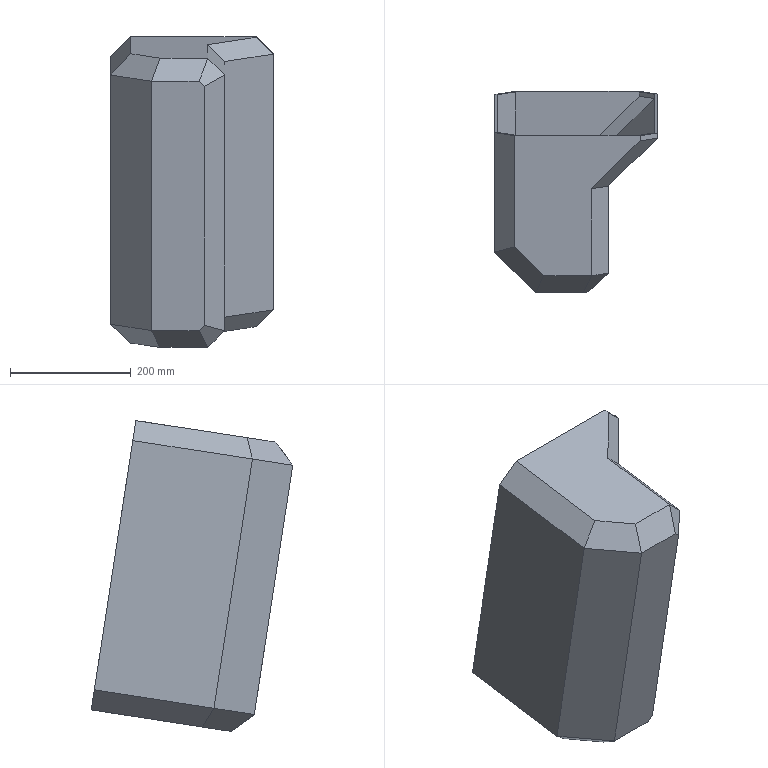Part | SolidWorks | features BaseBody 1 | 1 solid | 47 faces | box 269.204 x 333.071 x 514.026 mm | volume 1628567 mm3 | plane 47
STEP:
#1=CARTESIAN_POINT('',(-323.449,318.377,-419.092));
#2=VERTEX_POINT('',#1);
#3=CARTESIAN_POINT('',(-323.449,175.26,-441.176));
#4=VERTEX_POINT('',#3);
#5=CARTESIAN_POINT('',(-323.449,318.377,-419.092));
#6=DIRECTION('',(0.,-0.9883,-0.1525));
#7=VECTOR('',#6,1000.);
#8=LINE('',#5,#7);
#9=EDGE_CURVE('',#2,#4,#8,.T.);
#10=ORIENTED_EDGE('',*,*,#9,.F.);
#11=CARTESIAN_POINT('',(-352.149,314.001,-390.728));
#12=VERTEX_POINT('',#11);
#13=CARTESIAN_POINT('',(-323.449,318.377,-419.092));
#14=DIRECTION('',(-0.7071,-0.1078,0.6988));
#15=VECTOR('',#14,1000.);
#16=LINE('',#13,#15);
#17=EDGE_CURVE('',#2,#12,#16,.T.);
#18=ORIENTED_EDGE('',*,*,#17,.T.);
#19=CARTESIAN_POINT('',(-352.149,170.489,-412.872));
#20=VERTEX_POINT('',#19);
#21=CARTESIAN_POINT('',(-352.149,314.001,-390.728));
#22=DIRECTION('',(0.,-0.9883,-0.1525));
#23=VECTOR('',#22,1000.);
#24=LINE('',#21,#23);
#25=EDGE_CURVE('',#12,#20,#24,.T.);
#26=ORIENTED_EDGE('',*,*,#25,.T.);
#27=CARTESIAN_POINT('',(-351.829,170.222,-413.237));
#28=VERTEX_POINT('',#27);
#29=CARTESIAN_POINT('',(-352.149,170.489,-412.872));
#30=DIRECTION('',(0.5774,-0.4826,-0.6586));
#31=VECTOR('',#30,1000.);
#32=LINE('',#29,#31);
#33=EDGE_CURVE('',#20,#28,#32,.T.);
#34=ORIENTED_EDGE('',*,*,#33,.T.);
#35=CARTESIAN_POINT('',(-324.165,174.442,-440.577));
#36=VERTEX_POINT('',#35);
#37=CARTESIAN_POINT('',(-351.829,170.222,-413.237));
#38=DIRECTION('',(0.7071,0.1079,-0.6988));
#39=VECTOR('',#38,1000.);
#40=LINE('',#37,#39);
#41=EDGE_CURVE('',#28,#36,#40,.T.);
#42=ORIENTED_EDGE('',*,*,#41,.T.);
#43=CARTESIAN_POINT('',(-323.449,175.26,-441.176));
#44=DIRECTION('',(-0.5774,-0.6586,0.4826));
#45=VECTOR('',#44,1000.);
#46=LINE('',#43,#45);
#47=EDGE_CURVE('',#4,#36,#46,.T.);
#48=ORIENTED_EDGE('',*,*,#47,.F.);
#49=EDGE_LOOP('',(#10,#18,#26,#34,#42,#48));
#50=FACE_OUTER_BOUND('',#49,.T.);
#51=CARTESIAN_POINT('',(-363.649,121.114,-408.855));
#52=DIRECTION('',(-0.7071,0.1078,-0.6988));
#53=DIRECTION('',(-0.7029,0.,0.7113));
#54=AXIS2_PLACEMENT_3D('',#51,#52,#53);
#55=PLANE('',#54);
#56=ADVANCED_FACE('',(#50),#55,.F.);
#57=CARTESIAN_POINT('',(-324.165,239.716,-863.606));
#58=VERTEX_POINT('',#57);
#59=CARTESIAN_POINT('',(-323.449,240.315,-862.788));
#60=VERTEX_POINT('',#59);
#61=CARTESIAN_POINT('',(-324.165,239.716,-863.606));
#62=DIRECTION('',(0.5774,0.4826,0.6586));
#63=VECTOR('',#62,1000.);
#64=LINE('',#61,#63);
#65=EDGE_CURVE('',#58,#60,#64,.T.);
#66=ORIENTED_EDGE('',*,*,#65,.T.);
#67=CARTESIAN_POINT('',(-323.449,175.26,-441.176));
#68=DIRECTION('',(0.,0.1525,-0.9883));
#69=VECTOR('',#68,1000.);
#70=LINE('',#67,#69);
#71=EDGE_CURVE('',#4,#60,#70,.T.);
#72=ORIENTED_EDGE('',*,*,#71,.F.);
#73=ORIENTED_EDGE('',*,*,#47,.T.);
#74=CARTESIAN_POINT('',(-357.348,143.81,-459.65));
#75=VERTEX_POINT('',#74);
#76=CARTESIAN_POINT('',(-357.348,143.81,-459.65));
#77=DIRECTION('',(0.6769,0.6249,0.3891));
#78=VECTOR('',#77,1000.);
#79=LINE('',#76,#78);
#80=EDGE_CURVE('',#75,#36,#79,.T.);
#81=ORIENTED_EDGE('',*,*,#80,.F.);
#82=CARTESIAN_POINT('',(-357.348,204.76,-854.653));
#83=VERTEX_POINT('',#82);
#84=CARTESIAN_POINT('',(-357.348,204.76,-854.653));
#85=DIRECTION('',(0.,-0.1525,0.9883));
#86=VECTOR('',#85,1000.);
#87=LINE('',#84,#86);
#88=EDGE_CURVE('',#83,#75,#87,.T.);
#89=ORIENTED_EDGE('',*,*,#88,.F.);
#90=CARTESIAN_POINT('',(-357.348,204.76,-854.653));
#91=DIRECTION('',(0.6769,0.7131,-0.1826));
#92=VECTOR('',#91,1000.);
#93=LINE('',#90,#92);
#94=EDGE_CURVE('',#83,#58,#93,.T.);
#95=ORIENTED_EDGE('',*,*,#94,.T.);
#96=EDGE_LOOP('',(#66,#72,#73,#81,#89,#95));
#97=FACE_OUTER_BOUND('',#96,.T.);
#98=CARTESIAN_POINT('',(-321.336,164.858,-359.909));
#99=DIRECTION('',(-0.7071,0.6988,0.1078));
#100=DIRECTION('',(0.1508,0.,0.9886));
#101=AXIS2_PLACEMENT_3D('',#98,#99,#100);
#102=PLANE('',#101);
#103=ADVANCED_FACE('',(#97),#102,.F.);
#104=CARTESIAN_POINT('',(-366.009,206.081,-863.214));
#105=VERTEX_POINT('',#104);
#106=CARTESIAN_POINT('',(-351.829,243.933,-890.946));
#107=VERTEX_POINT('',#106);
#108=CARTESIAN_POINT('',(-366.009,206.081,-863.214));
#109=DIRECTION('',(0.2893,0.7722,-0.5657));
#110=VECTOR('',#109,1000.);
#111=LINE('',#108,#110);
#112=EDGE_CURVE('',#105,#107,#111,.T.);
#113=ORIENTED_EDGE('',*,*,#112,.T.);
#114=CARTESIAN_POINT('',(-324.165,239.716,-863.606));
#115=DIRECTION('',(-0.7071,0.1078,-0.6988));
#116=VECTOR('',#115,1000.);
#117=LINE('',#114,#116);
#118=EDGE_CURVE('',#58,#107,#117,.T.);
#119=ORIENTED_EDGE('',*,*,#118,.F.);
#120=ORIENTED_EDGE('',*,*,#94,.F.);
#121=CARTESIAN_POINT('',(-366.009,206.081,-863.214));
#122=DIRECTION('',(0.7071,-0.1078,0.6989));
#123=VECTOR('',#122,1000.);
#124=LINE('',#121,#123);
#125=EDGE_CURVE('',#105,#83,#124,.T.);
#126=ORIENTED_EDGE('',*,*,#125,.F.);
#127=EDGE_LOOP('',(#113,#119,#120,#126));
#128=FACE_OUTER_BOUND('',#127,.T.);
#129=CARTESIAN_POINT('',(-238.738,183.663,-734.28));
#130=DIRECTION('',(0.4977,-0.6262,-0.6002));
#131=DIRECTION('',(0.,0.692,-0.7219));
#132=AXIS2_PLACEMENT_3D('',#129,#130,#131);
#133=PLANE('',#132);
#134=ADVANCED_FACE('',(#128),#133,.T.);
#135=ORIENTED_EDGE('',*,*,#88,.T.);
#136=CARTESIAN_POINT('',(-366.009,142.489,-451.089));
#137=VERTEX_POINT('',#136);
#138=CARTESIAN_POINT('',(-357.348,143.81,-459.65));
#139=DIRECTION('',(-0.7071,-0.1078,0.6989));
#140=VECTOR('',#139,1000.);
#141=LINE('',#138,#140);
#142=EDGE_CURVE('',#75,#137,#141,.T.);
#143=ORIENTED_EDGE('',*,*,#142,.T.);
#144=CARTESIAN_POINT('',(-444.924,142.489,-451.089));
#145=VERTEX_POINT('',#144);
#146=CARTESIAN_POINT('',(-444.924,142.489,-451.089));
#147=DIRECTION('',(1.,0.,0.));
#148=VECTOR('',#147,1000.);
#149=LINE('',#146,#148);
#150=EDGE_CURVE('',#145,#137,#149,.T.);
#151=ORIENTED_EDGE('',*,*,#150,.F.);
#152=CARTESIAN_POINT('',(-444.924,206.081,-863.214));
#153=VERTEX_POINT('',#152);
#154=CARTESIAN_POINT('',(-444.924,142.489,-451.089));
#155=DIRECTION('',(0.,0.1525,-0.9883));
#156=VECTOR('',#155,1000.);
#157=LINE('',#154,#156);
#158=EDGE_CURVE('',#145,#153,#157,.T.);
#159=ORIENTED_EDGE('',*,*,#158,.T.);
#160=CARTESIAN_POINT('',(-366.009,206.081,-863.214));
#161=DIRECTION('',(-1.,0.,0.));
#162=VECTOR('',#161,1000.);
#163=LINE('',#160,#162);
#164=EDGE_CURVE('',#105,#153,#163,.T.);
#165=ORIENTED_EDGE('',*,*,#164,.F.);
#166=ORIENTED_EDGE('',*,*,#125,.T.);
#167=EDGE_LOOP('',(#135,#143,#151,#159,#165,#166));
#168=FACE_OUTER_BOUND('',#167,.T.);
#169=CARTESIAN_POINT('',(-335.294,177.166,-675.82));
#170=DIRECTION('',(0.,0.9883,0.1525));
#171=DIRECTION('',(1.,0.,0.));
#172=AXIS2_PLACEMENT_3D('',#169,#170,#171);
#173=PLANE('',#172);
#174=ADVANCED_FACE('',(#168),#173,.F.);
#175=ORIENTED_EDGE('',*,*,#164,.T.);
#176=CARTESIAN_POINT('',(-431.048,244.298,-891.213));
#177=VERTEX_POINT('',#176);
#178=CARTESIAN_POINT('',(-431.048,244.298,-891.213));
#179=DIRECTION('',(-0.2811,-0.7741,0.5672));
#180=VECTOR('',#179,1000.);
#181=LINE('',#178,#180);
#182=EDGE_CURVE('',#177,#153,#181,.T.);
#183=ORIENTED_EDGE('',*,*,#182,.F.);
#184=CARTESIAN_POINT('',(-352.149,244.298,-891.213));
#185=VERTEX_POINT('',#184);
#186=CARTESIAN_POINT('',(-431.048,244.298,-891.213));
#187=DIRECTION('',(1.,0.,0.));
#188=VECTOR('',#187,1000.);
#189=LINE('',#186,#188);
#190=EDGE_CURVE('',#177,#185,#189,.T.);
#191=ORIENTED_EDGE('',*,*,#190,.T.);
#192=CARTESIAN_POINT('',(-352.149,244.298,-891.213));
#193=DIRECTION('',(0.5774,-0.6586,0.4826));
#194=VECTOR('',#193,1000.);
#195=LINE('',#192,#194);
#196=EDGE_CURVE('',#185,#107,#195,.T.);
#197=ORIENTED_EDGE('',*,*,#196,.T.);
#198=ORIENTED_EDGE('',*,*,#112,.F.);
#199=EDGE_LOOP('',(#175,#183,#191,#197,#198));
#200=FACE_OUTER_BOUND('',#199,.T.);
#201=CARTESIAN_POINT('',(-444.924,206.081,-863.214));
#202=DIRECTION('',(0.,-0.591,-0.8067));
#203=DIRECTION('',(0.,-0.8067,0.591));
#204=AXIS2_PLACEMENT_3D('',#201,#202,#203);
#205=PLANE('',#204);
#206=ADVANCED_FACE('',(#200),#205,.T.);
#207=CARTESIAN_POINT('',(-352.149,387.809,-869.069));
#208=VERTEX_POINT('',#207);
#209=CARTESIAN_POINT('',(-352.149,244.298,-891.213));
#210=DIRECTION('',(0.,0.9883,0.1525));
#211=VECTOR('',#210,1000.);
#212=LINE('',#209,#211);
#213=EDGE_CURVE('',#185,#208,#212,.T.);
#214=ORIENTED_EDGE('',*,*,#213,.T.);
#215=CARTESIAN_POINT('',(-323.449,383.433,-840.705));
#216=VERTEX_POINT('',#215);
#217=CARTESIAN_POINT('',(-323.449,383.433,-840.705));
#218=DIRECTION('',(-0.7071,0.1078,-0.6988));
#219=VECTOR('',#218,1000.);
#220=LINE('',#217,#219);
#221=EDGE_CURVE('',#216,#208,#220,.T.);
#222=ORIENTED_EDGE('',*,*,#221,.F.);
#223=CARTESIAN_POINT('',(-323.449,383.433,-840.705));
#224=DIRECTION('',(0.,-0.9883,-0.1525));
#225=VECTOR('',#224,1000.);
#226=LINE('',#223,#225);
#227=EDGE_CURVE('',#216,#60,#226,.T.);
#228=ORIENTED_EDGE('',*,*,#227,.T.);
#229=ORIENTED_EDGE('',*,*,#65,.F.);
#230=ORIENTED_EDGE('',*,*,#118,.T.);
#231=ORIENTED_EDGE('',*,*,#196,.F.);
#232=EDGE_LOOP('',(#214,#222,#228,#229,#230,#231));
#233=FACE_OUTER_BOUND('',#232,.T.);
#234=CARTESIAN_POINT('',(-363.649,198.431,-909.927));
#235=DIRECTION('',(0.7071,0.1078,-0.6988));
#236=DIRECTION('',(0.,-0.9883,-0.1525));
#237=AXIS2_PLACEMENT_3D('',#234,#235,#236);
#238=PLANE('',#237);
#239=ADVANCED_FACE('',(#233),#238,.T.);
#240=ORIENTED_EDGE('',*,*,#227,.F.);
#241=CARTESIAN_POINT('',(-323.449,384.088,-841.185));
#242=VERTEX_POINT('',#241);
#243=CARTESIAN_POINT('',(-323.449,383.433,-840.705));
#244=DIRECTION('',(0.,0.8067,-0.591));
#245=VECTOR('',#244,1000.);
#246=LINE('',#243,#245);
#247=EDGE_CURVE('',#216,#242,#246,.T.);
#248=ORIENTED_EDGE('',*,*,#247,.T.);
#249=CARTESIAN_POINT('',(-323.449,318.857,-418.438));
#250=VERTEX_POINT('',#249);
#251=CARTESIAN_POINT('',(-323.449,384.088,-841.185));
#252=DIRECTION('',(0.,-0.1525,0.9883));
#253=VECTOR('',#252,1000.);
#254=LINE('',#251,#253);
#255=EDGE_CURVE('',#242,#250,#254,.T.);
#256=ORIENTED_EDGE('',*,*,#255,.T.);
#257=CARTESIAN_POINT('',(-323.449,318.377,-419.092));
#258=DIRECTION('',(0.,0.591,0.8067));
#259=VECTOR('',#258,1000.);
#260=LINE('',#257,#259);
#261=EDGE_CURVE('',#2,#250,#260,.T.);
#262=ORIENTED_EDGE('',*,*,#261,.F.);
#263=ORIENTED_EDGE('',*,*,#9,.T.);
#264=ORIENTED_EDGE('',*,*,#71,.T.);
#265=EDGE_LOOP('',(#240,#248,#256,#262,#263,#264));
#266=FACE_OUTER_BOUND('',#265,.T.);
#267=CARTESIAN_POINT('',(-323.449,142.123,-448.715));
#268=DIRECTION('',(1.,0.,0.));
#269=DIRECTION('',(0.,0.,-1.));
#270=AXIS2_PLACEMENT_3D('',#267,#268,#269);
#271=PLANE('',#270);
#272=ADVANCED_FACE('',(#266),#271,.T.);
#273=ORIENTED_EDGE('',*,*,#17,.F.);
#274=ORIENTED_EDGE('',*,*,#261,.T.);
#275=CARTESIAN_POINT('',(-243.823,397.552,-406.295));
#276=VERTEX_POINT('',#275);
#277=CARTESIAN_POINT('',(-243.823,397.552,-406.295));
#278=DIRECTION('',(-0.7071,-0.6988,-0.1078));
#279=VECTOR('',#278,1000.);
#280=LINE('',#277,#279);
#281=EDGE_CURVE('',#276,#250,#280,.T.);
#282=ORIENTED_EDGE('',*,*,#281,.F.);
#283=CARTESIAN_POINT('',(-271.949,393.263,-378.498));
#284=VERTEX_POINT('',#283);
#285=CARTESIAN_POINT('',(-243.823,397.552,-406.295));
#286=DIRECTION('',(-0.7071,-0.1078,0.6988));
#287=VECTOR('',#286,1000.);
#288=LINE('',#285,#287);
#289=EDGE_CURVE('',#276,#284,#288,.T.);
#290=ORIENTED_EDGE('',*,*,#289,.T.);
#291=CARTESIAN_POINT('',(-352.149,314.001,-390.728));
#292=DIRECTION('',(0.7071,0.6988,0.1078));
#293=VECTOR('',#292,1000.);
#294=LINE('',#291,#293);
#295=EDGE_CURVE('',#12,#284,#294,.T.);
#296=ORIENTED_EDGE('',*,*,#295,.F.);
#297=EDGE_LOOP('',(#273,#274,#282,#290,#296));
#298=FACE_OUTER_BOUND('',#297,.T.);
#299=CARTESIAN_POINT('',(-266.874,377.279,-406.387));
#300=DIRECTION('',(0.5774,-0.6586,0.4826));
#301=DIRECTION('',(0.,-0.591,-0.8067));
#302=AXIS2_PLACEMENT_3D('',#299,#300,#301);
#303=PLANE('',#302);
#304=ADVANCED_FACE('',(#298),#303,.T.);
#305=ORIENTED_EDGE('',*,*,#25,.F.);
#306=ORIENTED_EDGE('',*,*,#295,.T.);
#307=CARTESIAN_POINT('',(-271.949,401.752,-377.188));
#308=VERTEX_POINT('',#307);
#309=CARTESIAN_POINT('',(-271.949,401.752,-377.188));
#310=DIRECTION('',(0.,-0.9883,-0.1525));
#311=VECTOR('',#310,1000.);
#312=LINE('',#309,#311);
#313=EDGE_CURVE('',#308,#284,#312,.T.);
#314=ORIENTED_EDGE('',*,*,#313,.F.);
#315=CARTESIAN_POINT('',(-478.952,401.752,-377.188));
#316=VERTEX_POINT('',#315);
#317=CARTESIAN_POINT('',(-271.949,401.752,-377.188));
#318=DIRECTION('',(-1.,0.,0.));
#319=VECTOR('',#318,1000.);
#320=LINE('',#317,#319);
#321=EDGE_CURVE('',#308,#316,#320,.T.);
#322=ORIENTED_EDGE('',*,*,#321,.T.);
#323=CARTESIAN_POINT('',(-478.952,217.834,-405.567));
#324=VERTEX_POINT('',#323);
#325=CARTESIAN_POINT('',(-478.952,401.752,-377.188));
#326=DIRECTION('',(0.,-0.9883,-0.1525));
#327=VECTOR('',#326,1000.);
#328=LINE('',#325,#327);
#329=EDGE_CURVE('',#316,#324,#328,.T.);
#330=ORIENTED_EDGE('',*,*,#329,.T.);
#331=CARTESIAN_POINT('',(-431.048,170.489,-412.872));
#332=VERTEX_POINT('',#331);
#333=CARTESIAN_POINT('',(-431.048,170.489,-412.872));
#334=DIRECTION('',(-0.7071,0.6988,0.1078));
#335=VECTOR('',#334,1000.);
#336=LINE('',#333,#335);
#337=EDGE_CURVE('',#332,#324,#336,.T.);
#338=ORIENTED_EDGE('',*,*,#337,.F.);
#339=CARTESIAN_POINT('',(-431.048,170.489,-412.872));
#340=DIRECTION('',(1.,0.,0.));
#341=VECTOR('',#340,1000.);
#342=LINE('',#339,#341);
#343=EDGE_CURVE('',#332,#20,#342,.T.);
#344=ORIENTED_EDGE('',*,*,#343,.T.);
#345=EDGE_LOOP('',(#305,#306,#314,#322,#330,#338,#344));
#346=FACE_OUTER_BOUND('',#345,.T.);
#347=CARTESIAN_POINT('',(-481.526,137.381,-417.981));
#348=DIRECTION('',(0.,-0.1525,0.9883));
#349=DIRECTION('',(-1.,0.,0.));
#350=AXIS2_PLACEMENT_3D('',#347,#348,#349);
#351=PLANE('',#350);
#352=ADVANCED_FACE('',(#346),#351,.T.);
#353=CARTESIAN_POINT('',(-366.009,142.489,-451.089));
#354=DIRECTION('',(0.2893,0.5657,0.7722));
#355=VECTOR('',#354,1000.);
#356=LINE('',#353,#355);
#357=EDGE_CURVE('',#137,#28,#356,.T.);
#358=ORIENTED_EDGE('',*,*,#357,.T.);
#359=ORIENTED_EDGE('',*,*,#33,.F.);
#360=ORIENTED_EDGE('',*,*,#343,.F.);
#361=CARTESIAN_POINT('',(-431.048,170.489,-412.872));
#362=DIRECTION('',(-0.2811,-0.5672,-0.7741));
#363=VECTOR('',#362,1000.);
#364=LINE('',#361,#363);
#365=EDGE_CURVE('',#332,#145,#364,.T.);
#366=ORIENTED_EDGE('',*,*,#365,.T.);
#367=ORIENTED_EDGE('',*,*,#150,.T.);
#368=EDGE_LOOP('',(#358,#359,#360,#366,#367));
#369=FACE_OUTER_BOUND('',#368,.T.);
#370=CARTESIAN_POINT('',(-444.924,142.489,-451.089));
#371=DIRECTION('',(0.,0.8067,-0.591));
#372=DIRECTION('',(-1.,0.,0.));
#373=AXIS2_PLACEMENT_3D('',#370,#371,#372);
#374=PLANE('',#373);
#375=ADVANCED_FACE('',(#369),#374,.F.);
#376=CARTESIAN_POINT('',(-512.452,209.228,-440.791));
#377=VERTEX_POINT('',#376);
#378=CARTESIAN_POINT('',(-478.952,217.834,-405.567));
#379=DIRECTION('',(-0.6786,-0.1743,-0.7135));
#380=VECTOR('',#379,1000.);
#381=LINE('',#378,#380);
#382=EDGE_CURVE('',#324,#377,#381,.T.);
#383=ORIENTED_EDGE('',*,*,#382,.T.);
#384=CARTESIAN_POINT('',(-512.452,209.228,-440.791));
#385=DIRECTION('',(0.7071,-0.6988,-0.1078));
#386=VECTOR('',#385,1000.);
#387=LINE('',#384,#386);
#388=EDGE_CURVE('',#377,#145,#387,.T.);
#389=ORIENTED_EDGE('',*,*,#388,.T.);
#390=ORIENTED_EDGE('',*,*,#365,.F.);
#391=ORIENTED_EDGE('',*,*,#337,.T.);
#392=EDGE_LOOP('',(#383,#389,#390,#391));
#393=FACE_OUTER_BOUND('',#392,.T.);
#394=CARTESIAN_POINT('',(-512.452,209.228,-440.791));
#395=DIRECTION('',(0.5,0.602,-0.6226));
#396=DIRECTION('',(-0.7797,0.,-0.6262));
#397=AXIS2_PLACEMENT_3D('',#394,#395,#396);
#398=PLANE('',#397);
#399=ADVANCED_FACE('',(#393),#398,.F.);
#400=ORIENTED_EDGE('',*,*,#158,.F.);
#401=ORIENTED_EDGE('',*,*,#388,.F.);
#402=CARTESIAN_POINT('',(-512.452,272.82,-852.916));
#403=VERTEX_POINT('',#402);
#404=CARTESIAN_POINT('',(-512.452,209.228,-440.791));
#405=DIRECTION('',(0.,0.1525,-0.9883));
#406=VECTOR('',#405,1000.);
#407=LINE('',#404,#406);
#408=EDGE_CURVE('',#377,#403,#407,.T.);
#409=ORIENTED_EDGE('',*,*,#408,.T.);
#410=CARTESIAN_POINT('',(-512.452,272.82,-852.916));
#411=DIRECTION('',(0.7071,-0.6988,-0.1078));
#412=VECTOR('',#411,1000.);
#413=LINE('',#410,#412);
#414=EDGE_CURVE('',#403,#153,#413,.T.);
#415=ORIENTED_EDGE('',*,*,#414,.T.);
#416=EDGE_LOOP('',(#400,#401,#409,#415));
#417=FACE_OUTER_BOUND('',#416,.T.);
#418=CARTESIAN_POINT('',(-444.924,129.268,-365.4));
#419=DIRECTION('',(0.7071,0.6988,0.1078));
#420=DIRECTION('',(0.,0.1525,-0.9883));
#421=AXIS2_PLACEMENT_3D('',#418,#419,#420);
#422=PLANE('',#421);
#423=ADVANCED_FACE('',(#417),#422,.F.);
#424=ORIENTED_EDGE('',*,*,#182,.T.);
#425=ORIENTED_EDGE('',*,*,#414,.F.);
#426=CARTESIAN_POINT('',(-478.952,291.642,-883.908));
#427=VERTEX_POINT('',#426);
#428=CARTESIAN_POINT('',(-478.952,291.642,-883.908));
#429=DIRECTION('',(-0.6786,-0.3813,0.6278));
#430=VECTOR('',#429,1000.);
#431=LINE('',#428,#430);
#432=EDGE_CURVE('',#427,#403,#431,.T.);
#433=ORIENTED_EDGE('',*,*,#432,.F.);
#434=CARTESIAN_POINT('',(-478.952,291.642,-883.908));
#435=DIRECTION('',(0.7071,-0.6988,-0.1078));
#436=VECTOR('',#435,1000.);
#437=LINE('',#434,#436);
#438=EDGE_CURVE('',#427,#177,#437,.T.);
#439=ORIENTED_EDGE('',*,*,#438,.T.);
#440=EDGE_LOOP('',(#424,#425,#433,#439));
#441=FACE_OUTER_BOUND('',#440,.T.);
#442=CARTESIAN_POINT('',(-512.452,272.82,-852.916));
#443=DIRECTION('',(-0.5,-0.3863,-0.7751));
#444=DIRECTION('',(-0.8403,0.,0.5421));
#445=AXIS2_PLACEMENT_3D('',#442,#443,#444);
#446=PLANE('',#445);
#447=ADVANCED_FACE('',(#441),#446,.T.);
#448=ORIENTED_EDGE('',*,*,#213,.F.);
#449=ORIENTED_EDGE('',*,*,#190,.F.);
#450=ORIENTED_EDGE('',*,*,#438,.F.);
#451=CARTESIAN_POINT('',(-478.952,475.561,-855.529));
#452=VERTEX_POINT('',#451);
#453=CARTESIAN_POINT('',(-478.952,475.561,-855.529));
#454=DIRECTION('',(0.,-0.9883,-0.1525));
#455=VECTOR('',#454,1000.);
#456=LINE('',#453,#455);
#457=EDGE_CURVE('',#452,#427,#456,.T.);
#458=ORIENTED_EDGE('',*,*,#457,.F.);
#459=CARTESIAN_POINT('',(-271.949,475.561,-855.529));
#460=VERTEX_POINT('',#459);
#461=CARTESIAN_POINT('',(-478.952,475.561,-855.529));
#462=DIRECTION('',(1.,0.,0.));
#463=VECTOR('',#462,1000.);
#464=LINE('',#461,#463);
#465=EDGE_CURVE('',#452,#460,#464,.T.);
#466=ORIENTED_EDGE('',*,*,#465,.T.);
#467=CARTESIAN_POINT('',(-271.949,467.071,-856.839));
#468=VERTEX_POINT('',#467);
#469=CARTESIAN_POINT('',(-271.949,475.561,-855.529));
#470=DIRECTION('',(0.,-0.9883,-0.1525));
#471=VECTOR('',#470,1000.);
#472=LINE('',#469,#471);
#473=EDGE_CURVE('',#460,#468,#472,.T.);
#474=ORIENTED_EDGE('',*,*,#473,.T.);
#475=CARTESIAN_POINT('',(-352.149,387.809,-869.069));
#476=DIRECTION('',(0.7071,0.6988,0.1078));
#477=VECTOR('',#476,1000.);
#478=LINE('',#475,#477);
#479=EDGE_CURVE('',#208,#468,#478,.T.);
#480=ORIENTED_EDGE('',*,*,#479,.F.);
#481=EDGE_LOOP('',(#448,#449,#450,#458,#466,#474,#480));
#482=FACE_OUTER_BOUND('',#481,.T.);
#483=CARTESIAN_POINT('',(-269.545,211.19,-896.322));
#484=DIRECTION('',(0.,0.1525,-0.9883));
#485=DIRECTION('',(-1.,0.,0.));
#486=AXIS2_PLACEMENT_3D('',#483,#484,#485);
#487=PLANE('',#486);
#488=ADVANCED_FACE('',(#482),#487,.T.);
#489=CARTESIAN_POINT('',(-243.823,462.782,-829.042));
#490=VERTEX_POINT('',#489);
#491=CARTESIAN_POINT('',(-243.823,462.782,-829.042));
#492=DIRECTION('',(-0.7071,0.1078,-0.6988));
#493=VECTOR('',#492,1000.);
#494=LINE('',#491,#493);
#495=EDGE_CURVE('',#490,#468,#494,.T.);
#496=ORIENTED_EDGE('',*,*,#495,.F.);
#497=CARTESIAN_POINT('',(-323.449,384.088,-841.185));
#498=DIRECTION('',(0.7071,0.6988,0.1078));
#499=VECTOR('',#498,1000.);
#500=LINE('',#497,#499);
#501=EDGE_CURVE('',#242,#490,#500,.T.);
#502=ORIENTED_EDGE('',*,*,#501,.F.);
#503=ORIENTED_EDGE('',*,*,#247,.F.);
#504=ORIENTED_EDGE('',*,*,#221,.T.);
#505=ORIENTED_EDGE('',*,*,#479,.T.);
#506=EDGE_LOOP('',(#496,#502,#503,#504,#505));
#507=FACE_OUTER_BOUND('',#506,.T.);
#508=CARTESIAN_POINT('',(-266.874,443.424,-835.066));
#509=DIRECTION('',(-0.5774,0.4826,0.6586));
#510=DIRECTION('',(0.6413,0.7673,0.));
#511=AXIS2_PLACEMENT_3D('',#508,#509,#510);
#512=PLANE('',#511);
#513=ADVANCED_FACE('',(#507),#512,.F.);
#514=ORIENTED_EDGE('',*,*,#255,.F.);
#515=ORIENTED_EDGE('',*,*,#501,.T.);
#516=CARTESIAN_POINT('',(-243.249,463.262,-828.387));
#517=VERTEX_POINT('',#516);
#518=CARTESIAN_POINT('',(-243.823,462.782,-829.042));
#519=DIRECTION('',(0.5774,0.4826,0.6586));
#520=VECTOR('',#519,1000.);
#521=LINE('',#518,#520);
#522=EDGE_CURVE('',#490,#517,#521,.T.);
#523=ORIENTED_EDGE('',*,*,#522,.T.);
#524=CARTESIAN_POINT('',(-243.249,398.207,-406.775));
#525=VERTEX_POINT('',#524);
#526=CARTESIAN_POINT('',(-243.249,463.262,-828.387));
#527=DIRECTION('',(0.,-0.1525,0.9883));
#528=VECTOR('',#527,1000.);
#529=LINE('',#526,#528);
#530=EDGE_CURVE('',#517,#525,#529,.T.);
#531=ORIENTED_EDGE('',*,*,#530,.T.);
#532=CARTESIAN_POINT('',(-243.823,397.552,-406.295));
#533=DIRECTION('',(0.5774,0.6586,-0.4826));
#534=VECTOR('',#533,1000.);
#535=LINE('',#532,#534);
#536=EDGE_CURVE('',#276,#525,#535,.T.);
#537=ORIENTED_EDGE('',*,*,#536,.F.);
#538=ORIENTED_EDGE('',*,*,#281,.T.);
#539=EDGE_LOOP('',(#514,#515,#523,#531,#537,#538));
#540=FACE_OUTER_BOUND('',#539,.T.);
#541=CARTESIAN_POINT('',(-207.981,426.533,-359.088));
#542=DIRECTION('',(-0.7071,0.6988,0.1078));
#543=DIRECTION('',(0.1508,0.,0.9886));
#544=AXIS2_PLACEMENT_3D('',#541,#542,#543);
#545=PLANE('',#544);
#546=ADVANCED_FACE('',(#540),#545,.F.);
#547=ORIENTED_EDGE('',*,*,#536,.T.);
#548=CARTESIAN_POINT('',(-243.249,406.129,-405.552));
#549=VERTEX_POINT('',#548);
#550=CARTESIAN_POINT('',(-243.249,406.129,-405.552));
#551=DIRECTION('',(0.,-0.9883,-0.1525));
#552=VECTOR('',#551,1000.);
#553=LINE('',#550,#552);
#554=EDGE_CURVE('',#549,#525,#553,.T.);
#555=ORIENTED_EDGE('',*,*,#554,.F.);
#556=CARTESIAN_POINT('',(-243.249,406.129,-405.552));
#557=DIRECTION('',(-0.7071,-0.1078,0.6988));
#558=VECTOR('',#557,1000.);
#559=LINE('',#556,#558);
#560=EDGE_CURVE('',#549,#308,#559,.T.);
#561=ORIENTED_EDGE('',*,*,#560,.T.);
#562=ORIENTED_EDGE('',*,*,#313,.T.);
#563=ORIENTED_EDGE('',*,*,#289,.F.);
#564=EDGE_LOOP('',(#547,#555,#561,#562,#563));
#565=FACE_OUTER_BOUND('',#564,.T.);
#566=CARTESIAN_POINT('',(-283.449,121.114,-408.855));
#567=DIRECTION('',(-0.7071,0.1078,-0.6988));
#568=DIRECTION('',(-0.7029,0.,0.7113));
#569=AXIS2_PLACEMENT_3D('',#566,#567,#568);
#570=PLANE('',#569);
#571=ADVANCED_FACE('',(#565),#570,.F.);
#572=CARTESIAN_POINT('',(-273.606,402.362,-381.141));
#573=VERTEX_POINT('',#572);
#574=CARTESIAN_POINT('',(-247.249,406.381,-407.19));
#575=VERTEX_POINT('',#574);
#576=CARTESIAN_POINT('',(-273.606,402.362,-381.141));
#577=DIRECTION('',(0.7071,0.1078,-0.6988));
#578=VECTOR('',#577,1000.);
#579=LINE('',#576,#578);
#580=EDGE_CURVE('',#573,#575,#579,.T.);
#581=ORIENTED_EDGE('',*,*,#580,.F.);
#582=CARTESIAN_POINT('',(-477.296,402.362,-381.141));
#583=VERTEX_POINT('',#582);
#584=CARTESIAN_POINT('',(-273.606,402.362,-381.141));
#585=DIRECTION('',(-1.,0.,0.));
#586=VECTOR('',#585,1000.);
#587=LINE('',#584,#586);
#588=EDGE_CURVE('',#573,#583,#587,.T.);
#589=ORIENTED_EDGE('',*,*,#588,.T.);
#590=CARTESIAN_POINT('',(-508.452,407.113,-411.934));
#591=VERTEX_POINT('',#590);
#592=CARTESIAN_POINT('',(-508.452,407.113,-411.934));
#593=DIRECTION('',(0.7071,-0.1078,0.6988));
#594=VECTOR('',#593,1000.);
#595=LINE('',#592,#594);
#596=EDGE_CURVE('',#591,#583,#595,.T.);
#597=ORIENTED_EDGE('',*,*,#596,.F.);
#598=CARTESIAN_POINT('',(-508.452,470.2,-820.784));
#599=VERTEX_POINT('',#598);
#600=CARTESIAN_POINT('',(-508.452,407.113,-411.934));
#601=DIRECTION('',(0.,0.1525,-0.9883));
#602=VECTOR('',#601,1000.);
#603=LINE('',#600,#602);
#604=EDGE_CURVE('',#591,#599,#603,.T.);
#605=ORIENTED_EDGE('',*,*,#604,.T.);
#606=CARTESIAN_POINT('',(-477.296,474.951,-851.576));
#607=VERTEX_POINT('',#606);
#608=CARTESIAN_POINT('',(-477.296,474.951,-851.576));
#609=DIRECTION('',(-0.7071,-0.1078,0.6988));
#610=VECTOR('',#609,1000.);
#611=LINE('',#608,#610);
#612=EDGE_CURVE('',#607,#599,#611,.T.);
#613=ORIENTED_EDGE('',*,*,#612,.F.);
#614=CARTESIAN_POINT('',(-273.606,474.951,-851.576));
#615=VERTEX_POINT('',#614);
#616=CARTESIAN_POINT('',(-477.296,474.951,-851.576));
#617=DIRECTION('',(1.,0.,0.));
#618=VECTOR('',#617,1000.);
#619=LINE('',#616,#618);
#620=EDGE_CURVE('',#607,#615,#619,.T.);
#621=ORIENTED_EDGE('',*,*,#620,.T.);
#622=CARTESIAN_POINT('',(-247.249,470.932,-825.527));
#623=VERTEX_POINT('',#622);
#624=CARTESIAN_POINT('',(-247.249,470.932,-825.527));
#625=DIRECTION('',(-0.7071,0.1078,-0.6988));
#626=VECTOR('',#625,1000.);
#627=LINE('',#624,#626);
#628=EDGE_CURVE('',#623,#615,#627,.T.);
#629=ORIENTED_EDGE('',*,*,#628,.F.);
#630=CARTESIAN_POINT('',(-247.249,470.932,-825.527));
#631=DIRECTION('',(0.,-0.1525,0.9883));
#632=VECTOR('',#631,1000.);
#633=LINE('',#630,#632);
#634=EDGE_CURVE('',#623,#575,#633,.T.);
#635=ORIENTED_EDGE('',*,*,#634,.T.);
#636=EDGE_LOOP('',(#581,#589,#597,#605,#613,#621,#629,#635));
#637=FACE_BOUND('',#636,.T.);
#638=CARTESIAN_POINT('',(-512.452,406.861,-410.296));
#639=VERTEX_POINT('',#638);
#640=CARTESIAN_POINT('',(-512.452,470.452,-822.421));
#641=VERTEX_POINT('',#640);
#642=CARTESIAN_POINT('',(-512.452,406.861,-410.296));
#643=DIRECTION('',(0.,0.1525,-0.9883));
#644=VECTOR('',#643,1000.);
#645=LINE('',#642,#644);
#646=EDGE_CURVE('',#639,#641,#645,.T.);
#647=ORIENTED_EDGE('',*,*,#646,.F.);
#648=CARTESIAN_POINT('',(-478.952,401.752,-377.188));
#649=DIRECTION('',(-0.7071,0.1078,-0.6988));
#650=VECTOR('',#649,1000.);
#651=LINE('',#648,#650);
#652=EDGE_CURVE('',#316,#639,#651,.T.);
#653=ORIENTED_EDGE('',*,*,#652,.F.);
#654=ORIENTED_EDGE('',*,*,#321,.F.);
#655=ORIENTED_EDGE('',*,*,#560,.F.);
#656=CARTESIAN_POINT('',(-243.249,471.184,-827.165));
#657=VERTEX_POINT('',#656);
#658=CARTESIAN_POINT('',(-243.249,471.184,-827.165));
#659=DIRECTION('',(0.,-0.1525,0.9883));
#660=VECTOR('',#659,1000.);
#661=LINE('',#658,#660);
#662=EDGE_CURVE('',#657,#549,#661,.T.);
#663=ORIENTED_EDGE('',*,*,#662,.F.);
#664=CARTESIAN_POINT('',(-271.949,475.561,-855.529));
#665=DIRECTION('',(0.7071,-0.1078,0.6988));
#666=VECTOR('',#665,1000.);
#667=LINE('',#664,#666);
#668=EDGE_CURVE('',#460,#657,#667,.T.);
#669=ORIENTED_EDGE('',*,*,#668,.F.);
#670=ORIENTED_EDGE('',*,*,#465,.F.);
#671=CARTESIAN_POINT('',(-512.452,470.452,-822.421));
#672=DIRECTION('',(0.7071,0.1078,-0.6988));
#673=VECTOR('',#672,1000.);
#674=LINE('',#671,#673);
#675=EDGE_CURVE('',#641,#452,#674,.T.);
#676=ORIENTED_EDGE('',*,*,#675,.F.);
#677=EDGE_LOOP('',(#647,#653,#654,#655,#663,#669,#670,#676));
#678=FACE_OUTER_BOUND('',#677,.T.);
#679=CARTESIAN_POINT('',(-335.294,441.537,-635.027));
#680=DIRECTION('',(0.,0.9883,0.1525));
#681=DIRECTION('',(1.,0.,0.));
#682=AXIS2_PLACEMENT_3D('',#679,#680,#681);
#683=PLANE('',#682);
#684=ADVANCED_FACE('',(#637,#678),#683,.T.);
#685=CARTESIAN_POINT('',(-512.452,470.452,-822.421));
#686=DIRECTION('',(0.,-0.9883,-0.1525));
#687=VECTOR('',#686,1000.);
#688=LINE('',#685,#687);
#689=EDGE_CURVE('',#641,#403,#688,.T.);
#690=ORIENTED_EDGE('',*,*,#689,.F.);
#691=ORIENTED_EDGE('',*,*,#675,.T.);
#692=ORIENTED_EDGE('',*,*,#457,.T.);
#693=ORIENTED_EDGE('',*,*,#432,.T.);
#694=EDGE_LOOP('',(#690,#691,#692,#693));
#695=FACE_OUTER_BOUND('',#694,.T.);
#696=CARTESIAN_POINT('',(-512.452,191.568,-865.453));
#697=DIRECTION('',(-0.7071,0.1078,-0.6988));
#698=DIRECTION('',(-0.7029,0.,0.7113));
#699=AXIS2_PLACEMENT_3D('',#696,#697,#698);
#700=PLANE('',#699);
#701=ADVANCED_FACE('',(#695),#700,.T.);
#702=ORIENTED_EDGE('',*,*,#408,.F.);
#703=CARTESIAN_POINT('',(-512.452,406.861,-410.296));
#704=DIRECTION('',(0.,-0.9883,-0.1525));
#705=VECTOR('',#704,1000.);
#706=LINE('',#703,#705);
#707=EDGE_CURVE('',#639,#377,#706,.T.);
#708=ORIENTED_EDGE('',*,*,#707,.F.);
#709=ORIENTED_EDGE('',*,*,#646,.T.);
#710=ORIENTED_EDGE('',*,*,#689,.T.);
#711=EDGE_LOOP('',(#702,#708,#709,#710));
#712=FACE_OUTER_BOUND('',#711,.T.);
#713=CARTESIAN_POINT('',(-512.452,206.474,-865.759));
#714=DIRECTION('',(-1.,0.,0.));
#715=DIRECTION('',(0.,1.,0.));
#716=AXIS2_PLACEMENT_3D('',#713,#714,#715);
#717=PLANE('',#716);
#718=ADVANCED_FACE('',(#712),#717,.T.);
#719=ORIENTED_EDGE('',*,*,#329,.F.);
#720=ORIENTED_EDGE('',*,*,#652,.T.);
#721=ORIENTED_EDGE('',*,*,#707,.T.);
#722=ORIENTED_EDGE('',*,*,#382,.F.);
#723=EDGE_LOOP('',(#719,#720,#721,#722));
#724=FACE_OUTER_BOUND('',#723,.T.);
#725=CARTESIAN_POINT('',(-512.452,127.977,-453.328));
#726=DIRECTION('',(0.7071,0.1078,-0.6988));
#727=DIRECTION('',(0.,-0.9883,-0.1525));
#728=AXIS2_PLACEMENT_3D('',#725,#726,#727);
#729=PLANE('',#728);
#730=ADVANCED_FACE('',(#724),#729,.F.);
#731=ORIENTED_EDGE('',*,*,#473,.F.);
#732=ORIENTED_EDGE('',*,*,#668,.T.);
#733=CARTESIAN_POINT('',(-243.249,471.184,-827.165));
#734=DIRECTION('',(0.,-0.9883,-0.1525));
#735=VECTOR('',#734,1000.);
#736=LINE('',#733,#735);
#737=EDGE_CURVE('',#657,#517,#736,.T.);
#738=ORIENTED_EDGE('',*,*,#737,.T.);
#739=ORIENTED_EDGE('',*,*,#522,.F.);
#740=ORIENTED_EDGE('',*,*,#495,.T.);
#741=EDGE_LOOP('',(#731,#732,#738,#739,#740));
#742=FACE_OUTER_BOUND('',#741,.T.);
#743=CARTESIAN_POINT('',(-283.449,198.431,-909.927));
#744=DIRECTION('',(0.7071,0.1078,-0.6988));
#745=DIRECTION('',(0.,-0.9883,-0.1525));
#746=AXIS2_PLACEMENT_3D('',#743,#744,#745);
#747=PLANE('',#746);
#748=ADVANCED_FACE('',(#742),#747,.T.);
#749=ORIENTED_EDGE('',*,*,#530,.F.);
#750=ORIENTED_EDGE('',*,*,#737,.F.);
#751=ORIENTED_EDGE('',*,*,#662,.T.);
#752=ORIENTED_EDGE('',*,*,#554,.T.);
#753=EDGE_LOOP('',(#749,#750,#751,#752));
#754=FACE_OUTER_BOUND('',#753,.T.);
#755=CARTESIAN_POINT('',(-243.249,142.123,-448.715));
#756=DIRECTION('',(1.,0.,0.));
#757=DIRECTION('',(0.,0.,-1.));
#758=AXIS2_PLACEMENT_3D('',#755,#756,#757);
#759=PLANE('',#758);
#760=ADVANCED_FACE('',(#754),#759,.T.);
#761=CARTESIAN_POINT('',(-247.249,464.647,-826.497));
#762=VERTEX_POINT('',#761);
#763=CARTESIAN_POINT('',(-247.249,470.932,-825.527));
#764=DIRECTION('',(0.,-0.9883,-0.1525));
#765=VECTOR('',#764,1000.);
#766=LINE('',#763,#765);
#767=EDGE_CURVE('',#623,#762,#766,.T.);
#768=ORIENTED_EDGE('',*,*,#767,.T.);
#769=CARTESIAN_POINT('',(-247.249,400.097,-408.159));
#770=VERTEX_POINT('',#769);
#771=CARTESIAN_POINT('',(-247.249,464.647,-826.497));
#772=DIRECTION('',(0.,-0.1525,0.9883));
#773=VECTOR('',#772,1000.);
#774=LINE('',#771,#773);
#775=EDGE_CURVE('',#762,#770,#774,.T.);
#776=ORIENTED_EDGE('',*,*,#775,.T.);
#777=CARTESIAN_POINT('',(-247.249,406.381,-407.19));
#778=DIRECTION('',(0.,-0.9883,-0.1525));
#779=VECTOR('',#778,1000.);
#780=LINE('',#777,#779);
#781=EDGE_CURVE('',#575,#770,#780,.T.);
#782=ORIENTED_EDGE('',*,*,#781,.F.);
#783=ORIENTED_EDGE('',*,*,#634,.F.);
#784=EDGE_LOOP('',(#768,#776,#782,#783));
#785=FACE_OUTER_BOUND('',#784,.T.);
#786=CARTESIAN_POINT('',(-247.249,142.123,-448.715));
#787=DIRECTION('',(1.,0.,0.));
#788=DIRECTION('',(0.,0.,-1.));
#789=AXIS2_PLACEMENT_3D('',#786,#787,#788);
#790=PLANE('',#789);
#791=ADVANCED_FACE('',(#785),#790,.F.);
#792=ORIENTED_EDGE('',*,*,#781,.T.);
#793=CARTESIAN_POINT('',(-248.208,399.002,-407.357));
#794=VERTEX_POINT('',#793);
#795=CARTESIAN_POINT('',(-247.249,400.097,-408.159));
#796=DIRECTION('',(-0.5774,-0.6586,0.4826));
#797=VECTOR('',#796,1000.);
#798=LINE('',#795,#797);
#799=EDGE_CURVE('',#770,#794,#798,.T.);
#800=ORIENTED_EDGE('',*,*,#799,.T.);
#801=CARTESIAN_POINT('',(-273.606,395.129,-382.257));
#802=VERTEX_POINT('',#801);
#803=CARTESIAN_POINT('',(-248.208,399.002,-407.357));
#804=DIRECTION('',(-0.7071,-0.1078,0.6988));
#805=VECTOR('',#804,1000.);
#806=LINE('',#803,#805);
#807=EDGE_CURVE('',#794,#802,#806,.T.);
#808=ORIENTED_EDGE('',*,*,#807,.T.);
#809=CARTESIAN_POINT('',(-273.606,402.362,-381.141));
#810=DIRECTION('',(0.,-0.9883,-0.1525));
#811=VECTOR('',#810,1000.);
#812=LINE('',#809,#811);
#813=EDGE_CURVE('',#573,#802,#812,.T.);
#814=ORIENTED_EDGE('',*,*,#813,.F.);
#815=ORIENTED_EDGE('',*,*,#580,.T.);
#816=EDGE_LOOP('',(#792,#800,#808,#814,#815));
#817=FACE_OUTER_BOUND('',#816,.T.);
#818=CARTESIAN_POINT('',(-286.277,121.546,-411.65));
#819=DIRECTION('',(-0.7071,0.1078,-0.6988));
#820=DIRECTION('',(-0.7029,0.,0.7113));
#821=AXIS2_PLACEMENT_3D('',#818,#819,#820);
#822=PLANE('',#821);
#823=ADVANCED_FACE('',(#817),#822,.T.);
#824=ORIENTED_EDGE('',*,*,#813,.T.);
#825=CARTESIAN_POINT('',(-353.806,315.867,-394.487));
#826=VERTEX_POINT('',#825);
#827=CARTESIAN_POINT('',(-353.806,315.867,-394.487));
#828=DIRECTION('',(0.7071,0.6988,0.1078));
#829=VECTOR('',#828,1000.);
#830=LINE('',#827,#829);
#831=EDGE_CURVE('',#826,#802,#830,.T.);
#832=ORIENTED_EDGE('',*,*,#831,.F.);
#833=CARTESIAN_POINT('',(-353.806,172.736,-416.573));
#834=VERTEX_POINT('',#833);
#835=CARTESIAN_POINT('',(-353.806,315.867,-394.487));
#836=DIRECTION('',(0.,-0.9883,-0.1525));
#837=VECTOR('',#836,1000.);
#838=LINE('',#835,#837);
#839=EDGE_CURVE('',#826,#834,#838,.T.);
#840=ORIENTED_EDGE('',*,*,#839,.T.);
#841=CARTESIAN_POINT('',(-430.361,172.736,-416.573));
#842=VERTEX_POINT('',#841);
#843=CARTESIAN_POINT('',(-430.361,172.736,-416.573));
#844=DIRECTION('',(1.,0.,0.));
#845=VECTOR('',#844,1000.);
#846=LINE('',#843,#845);
#847=EDGE_CURVE('',#842,#834,#846,.T.);
#848=ORIENTED_EDGE('',*,*,#847,.F.);
#849=CARTESIAN_POINT('',(-477.296,219.122,-409.415));
#850=VERTEX_POINT('',#849);
#851=CARTESIAN_POINT('',(-477.296,219.122,-409.415));
#852=DIRECTION('',(0.7071,-0.6988,-0.1078));
#853=VECTOR('',#852,1000.);
#854=LINE('',#851,#853);
#855=EDGE_CURVE('',#850,#842,#854,.T.);
#856=ORIENTED_EDGE('',*,*,#855,.F.);
#857=CARTESIAN_POINT('',(-477.296,402.362,-381.141));
#858=DIRECTION('',(0.,-0.9883,-0.1525));
#859=VECTOR('',#858,1000.);
#860=LINE('',#857,#859);
#861=EDGE_CURVE('',#583,#850,#860,.T.);
#862=ORIENTED_EDGE('',*,*,#861,.F.);
#863=ORIENTED_EDGE('',*,*,#588,.F.);
#864=EDGE_LOOP('',(#824,#832,#840,#848,#856,#862,#863));
#865=FACE_OUTER_BOUND('',#864,.T.);
#866=CARTESIAN_POINT('',(-481.526,137.991,-421.934));
#867=DIRECTION('',(0.,-0.1525,0.9883));
#868=DIRECTION('',(-1.,0.,0.));
#869=AXIS2_PLACEMENT_3D('',#866,#867,#868);
#870=PLANE('',#869);
#871=ADVANCED_FACE('',(#865),#870,.F.);
#872=ORIENTED_EDGE('',*,*,#861,.T.);
#873=CARTESIAN_POINT('',(-508.452,211.118,-442.176));
#874=VERTEX_POINT('',#873);
#875=CARTESIAN_POINT('',(-477.296,219.122,-409.415));
#876=DIRECTION('',(-0.6786,-0.1743,-0.7135));
#877=VECTOR('',#876,1000.);
#878=LINE('',#875,#877);
#879=EDGE_CURVE('',#850,#874,#878,.T.);
#880=ORIENTED_EDGE('',*,*,#879,.T.);
#881=CARTESIAN_POINT('',(-508.452,407.113,-411.934));
#882=DIRECTION('',(0.,-0.9883,-0.1525));
#883=VECTOR('',#882,1000.);
#884=LINE('',#881,#883);
#885=EDGE_CURVE('',#591,#874,#884,.T.);
#886=ORIENTED_EDGE('',*,*,#885,.F.);
#887=ORIENTED_EDGE('',*,*,#596,.T.);
#888=EDGE_LOOP('',(#872,#880,#886,#887));
#889=FACE_OUTER_BOUND('',#888,.T.);
#890=CARTESIAN_POINT('',(-509.624,128.408,-456.124));
#891=DIRECTION('',(0.7071,0.1078,-0.6988));
#892=DIRECTION('',(0.,-0.9883,-0.1525));
#893=AXIS2_PLACEMENT_3D('',#890,#891,#892);
#894=PLANE('',#893);
#895=ADVANCED_FACE('',(#889),#894,.T.);
#896=ORIENTED_EDGE('',*,*,#885,.T.);
#897=CARTESIAN_POINT('',(-508.452,274.205,-851.026));
#898=VERTEX_POINT('',#897);
#899=CARTESIAN_POINT('',(-508.452,211.118,-442.176));
#900=DIRECTION('',(0.,0.1525,-0.9883));
#901=VECTOR('',#900,1000.);
#902=LINE('',#899,#901);
#903=EDGE_CURVE('',#874,#898,#902,.T.);
#904=ORIENTED_EDGE('',*,*,#903,.T.);
#905=CARTESIAN_POINT('',(-508.452,470.2,-820.784));
#906=DIRECTION('',(0.,-0.9883,-0.1525));
#907=VECTOR('',#906,1000.);
#908=LINE('',#905,#907);
#909=EDGE_CURVE('',#599,#898,#908,.T.);
#910=ORIENTED_EDGE('',*,*,#909,.F.);
#911=ORIENTED_EDGE('',*,*,#604,.F.);
#912=EDGE_LOOP('',(#896,#904,#910,#911));
#913=FACE_OUTER_BOUND('',#912,.T.);
#914=CARTESIAN_POINT('',(-508.452,206.474,-865.759));
#915=DIRECTION('',(-1.,0.,0.));
#916=DIRECTION('',(0.,1.,0.));
#917=AXIS2_PLACEMENT_3D('',#914,#915,#916);
#918=PLANE('',#917);
#919=ADVANCED_FACE('',(#913),#918,.F.);
#920=ORIENTED_EDGE('',*,*,#909,.T.);
#921=CARTESIAN_POINT('',(-477.296,291.711,-879.85));
#922=VERTEX_POINT('',#921);
#923=CARTESIAN_POINT('',(-477.296,291.711,-879.85));
#924=DIRECTION('',(-0.6786,-0.3813,0.6278));
#925=VECTOR('',#924,1000.);
#926=LINE('',#923,#925);
#927=EDGE_CURVE('',#922,#898,#926,.T.);
#928=ORIENTED_EDGE('',*,*,#927,.F.);
#929=CARTESIAN_POINT('',(-477.296,474.951,-851.576));
#930=DIRECTION('',(0.,-0.9883,-0.1525));
#931=VECTOR('',#930,1000.);
#932=LINE('',#929,#931);
#933=EDGE_CURVE('',#607,#922,#932,.T.);
#934=ORIENTED_EDGE('',*,*,#933,.F.);
#935=ORIENTED_EDGE('',*,*,#612,.T.);
#936=EDGE_LOOP('',(#920,#928,#934,#935));
#937=FACE_OUTER_BOUND('',#936,.T.);
#938=CARTESIAN_POINT('',(-509.624,191.137,-862.658));
#939=DIRECTION('',(-0.7071,0.1078,-0.6988));
#940=DIRECTION('',(-0.7029,0.,0.7113));
#941=AXIS2_PLACEMENT_3D('',#938,#939,#940);
#942=PLANE('',#941);
#943=ADVANCED_FACE('',(#937),#942,.F.);
#944=ORIENTED_EDGE('',*,*,#933,.T.);
#945=CARTESIAN_POINT('',(-430.361,245.325,-887.008));
#946=VERTEX_POINT('',#945);
#947=CARTESIAN_POINT('',(-430.361,245.325,-887.008));
#948=DIRECTION('',(-0.7071,0.6988,0.1078));
#949=VECTOR('',#948,1000.);
#950=LINE('',#947,#949);
#951=EDGE_CURVE('',#946,#922,#950,.T.);
#952=ORIENTED_EDGE('',*,*,#951,.F.);
#953=CARTESIAN_POINT('',(-353.806,245.325,-887.008));
#954=VERTEX_POINT('',#953);
#955=CARTESIAN_POINT('',(-430.361,245.325,-887.008));
#956=DIRECTION('',(1.,0.,0.));
#957=VECTOR('',#956,1000.);
#958=LINE('',#955,#957);
#959=EDGE_CURVE('',#946,#954,#958,.T.);
#960=ORIENTED_EDGE('',*,*,#959,.T.);
#961=CARTESIAN_POINT('',(-353.806,388.456,-864.922));
#962=VERTEX_POINT('',#961);
#963=CARTESIAN_POINT('',(-353.806,245.325,-887.008));
#964=DIRECTION('',(0.,0.9883,0.1525));
#965=VECTOR('',#964,1000.);
#966=LINE('',#963,#965);
#967=EDGE_CURVE('',#954,#962,#966,.T.);
#968=ORIENTED_EDGE('',*,*,#967,.T.);
#969=CARTESIAN_POINT('',(-273.606,467.718,-852.692));
#970=VERTEX_POINT('',#969);
#971=CARTESIAN_POINT('',(-353.806,388.456,-864.922));
#972=DIRECTION('',(0.7071,0.6988,0.1078));
#973=VECTOR('',#972,1000.);
#974=LINE('',#971,#973);
#975=EDGE_CURVE('',#962,#970,#974,.T.);
#976=ORIENTED_EDGE('',*,*,#975,.T.);
#977=CARTESIAN_POINT('',(-273.606,474.951,-851.576));
#978=DIRECTION('',(0.,-0.9883,-0.1525));
#979=VECTOR('',#978,1000.);
#980=LINE('',#977,#979);
#981=EDGE_CURVE('',#615,#970,#980,.T.);
#982=ORIENTED_EDGE('',*,*,#981,.F.);
#983=ORIENTED_EDGE('',*,*,#620,.F.);
#984=EDGE_LOOP('',(#944,#952,#960,#968,#976,#982,#983));
#985=FACE_OUTER_BOUND('',#984,.T.);
#986=CARTESIAN_POINT('',(-269.545,210.58,-892.369));
#987=DIRECTION('',(0.,0.1525,-0.9883));
#988=DIRECTION('',(-1.,0.,0.));
#989=AXIS2_PLACEMENT_3D('',#986,#987,#988);
#990=PLANE('',#989);
#991=ADVANCED_FACE('',(#985),#990,.F.);
#992=ORIENTED_EDGE('',*,*,#981,.T.);
#993=CARTESIAN_POINT('',(-248.208,463.845,-827.592));
#994=VERTEX_POINT('',#993);
#995=CARTESIAN_POINT('',(-248.208,463.845,-827.592));
#996=DIRECTION('',(-0.7071,0.1078,-0.6988));
#997=VECTOR('',#996,1000.);
#998=LINE('',#995,#997);
#999=EDGE_CURVE('',#994,#970,#998,.T.);
#1000=ORIENTED_EDGE('',*,*,#999,.F.);
#1001=CARTESIAN_POINT('',(-247.249,464.647,-826.497));
#1002=DIRECTION('',(-0.5774,-0.4826,-0.6586));
#1003=VECTOR('',#1002,1000.);
#1004=LINE('',#1001,#1003);
#1005=EDGE_CURVE('',#762,#994,#1004,.T.);
#1006=ORIENTED_EDGE('',*,*,#1005,.F.);
#1007=ORIENTED_EDGE('',*,*,#767,.F.);
#1008=ORIENTED_EDGE('',*,*,#628,.T.);
#1009=EDGE_LOOP('',(#992,#1000,#1006,#1007,#1008));
#1010=FACE_OUTER_BOUND('',#1009,.T.);
#1011=CARTESIAN_POINT('',(-286.277,197.999,-907.132));
#1012=DIRECTION('',(0.7071,0.1078,-0.6988));
#1013=DIRECTION('',(0.,-0.9883,-0.1525));
#1014=AXIS2_PLACEMENT_3D('',#1011,#1012,#1013);
#1015=PLANE('',#1014);
#1016=ADVANCED_FACE('',(#1010),#1015,.F.);
#1017=ORIENTED_EDGE('',*,*,#799,.F.);
#1018=ORIENTED_EDGE('',*,*,#775,.F.);
#1019=ORIENTED_EDGE('',*,*,#1005,.T.);
#1020=CARTESIAN_POINT('',(-327.449,385.531,-839.676));
#1021=VERTEX_POINT('',#1020);
#1022=CARTESIAN_POINT('',(-248.208,463.845,-827.592));
#1023=DIRECTION('',(-0.7071,-0.6988,-0.1078));
#1024=VECTOR('',#1023,1000.);
#1025=LINE('',#1022,#1024);
#1026=EDGE_CURVE('',#994,#1021,#1025,.T.);
#1027=ORIENTED_EDGE('',*,*,#1026,.T.);
#1028=CARTESIAN_POINT('',(-327.449,320.688,-419.441));
#1029=VERTEX_POINT('',#1028);
#1030=CARTESIAN_POINT('',(-327.449,385.531,-839.676));
#1031=DIRECTION('',(0.,-0.1525,0.9883));
#1032=VECTOR('',#1031,1000.);
#1033=LINE('',#1030,#1032);
#1034=EDGE_CURVE('',#1021,#1029,#1033,.T.);
#1035=ORIENTED_EDGE('',*,*,#1034,.T.);
#1036=CARTESIAN_POINT('',(-327.449,320.688,-419.441));
#1037=DIRECTION('',(0.7071,0.6988,0.1078));
#1038=VECTOR('',#1037,1000.);
#1039=LINE('',#1036,#1038);
#1040=EDGE_CURVE('',#1029,#794,#1039,.T.);
#1041=ORIENTED_EDGE('',*,*,#1040,.T.);
#1042=EDGE_LOOP('',(#1017,#1018,#1019,#1027,#1035,#1041));
#1043=FACE_OUTER_BOUND('',#1042,.T.);
#1044=CARTESIAN_POINT('',(-210.81,429.329,-358.656));
#1045=DIRECTION('',(-0.7071,0.6988,0.1078));
#1046=DIRECTION('',(0.1508,0.,0.9886));
#1047=AXIS2_PLACEMENT_3D('',#1044,#1045,#1046);
#1048=PLANE('',#1047);
#1049=ADVANCED_FACE('',(#1043),#1048,.T.);
#1050=ORIENTED_EDGE('',*,*,#807,.F.);
#1051=ORIENTED_EDGE('',*,*,#1040,.F.);
#1052=CARTESIAN_POINT('',(-327.449,319.886,-420.536));
#1053=VERTEX_POINT('',#1052);
#1054=CARTESIAN_POINT('',(-327.449,319.886,-420.536));
#1055=DIRECTION('',(0.,0.591,0.8067));
#1056=VECTOR('',#1055,1000.);
#1057=LINE('',#1054,#1056);
#1058=EDGE_CURVE('',#1053,#1029,#1057,.T.);
#1059=ORIENTED_EDGE('',*,*,#1058,.F.);
#1060=CARTESIAN_POINT('',(-327.449,319.886,-420.536));
#1061=DIRECTION('',(-0.7071,-0.1078,0.6988));
#1062=VECTOR('',#1061,1000.);
#1063=LINE('',#1060,#1062);
#1064=EDGE_CURVE('',#1053,#826,#1063,.T.);
#1065=ORIENTED_EDGE('',*,*,#1064,.T.);
#1066=ORIENTED_EDGE('',*,*,#831,.T.);
#1067=EDGE_LOOP('',(#1050,#1051,#1059,#1065,#1066));
#1068=FACE_OUTER_BOUND('',#1067,.T.);
#1069=CARTESIAN_POINT('',(-269.183,379.913,-408.317));
#1070=DIRECTION('',(0.5774,-0.6586,0.4826));
#1071=DIRECTION('',(0.,-0.591,-0.8067));
#1072=AXIS2_PLACEMENT_3D('',#1069,#1070,#1071);
#1073=PLANE('',#1072);
#1074=ADVANCED_FACE('',(#1068),#1073,.F.);
#1075=CARTESIAN_POINT('',(-353.497,172.478,-416.925));
#1076=VERTEX_POINT('',#1075);
#1077=CARTESIAN_POINT('',(-353.497,172.478,-416.925));
#1078=DIRECTION('',(-0.5774,0.4826,0.6586));
#1079=VECTOR('',#1078,1000.);
#1080=LINE('',#1077,#1079);
#1081=EDGE_CURVE('',#1076,#834,#1080,.T.);
#1082=ORIENTED_EDGE('',*,*,#1081,.T.);
#1083=ORIENTED_EDGE('',*,*,#839,.F.);
#1084=ORIENTED_EDGE('',*,*,#1064,.F.);
#1085=CARTESIAN_POINT('',(-327.449,177.15,-442.56));
#1086=VERTEX_POINT('',#1085);
#1087=CARTESIAN_POINT('',(-327.449,319.886,-420.536));
#1088=DIRECTION('',(0.,-0.9883,-0.1525));
#1089=VECTOR('',#1088,1000.);
#1090=LINE('',#1087,#1089);
#1091=EDGE_CURVE('',#1053,#1086,#1090,.T.);
#1092=ORIENTED_EDGE('',*,*,#1091,.T.);
#1093=CARTESIAN_POINT('',(-328.155,176.345,-441.97));
#1094=VERTEX_POINT('',#1093);
#1095=CARTESIAN_POINT('',(-328.155,176.345,-441.97));
#1096=DIRECTION('',(0.5774,0.6586,-0.4826));
#1097=VECTOR('',#1096,1000.);
#1098=LINE('',#1095,#1097);
#1099=EDGE_CURVE('',#1094,#1086,#1098,.T.);
#1100=ORIENTED_EDGE('',*,*,#1099,.F.);
#1101=CARTESIAN_POINT('',(-328.155,176.345,-441.97));
#1102=DIRECTION('',(-0.7071,-0.1079,0.6988));
#1103=VECTOR('',#1102,1000.);
#1104=LINE('',#1101,#1103);
#1105=EDGE_CURVE('',#1094,#1076,#1104,.T.);
#1106=ORIENTED_EDGE('',*,*,#1105,.T.);
#1107=EDGE_LOOP('',(#1082,#1083,#1084,#1092,#1100,#1106));
#1108=FACE_OUTER_BOUND('',#1107,.T.);
#1109=CARTESIAN_POINT('',(-366.477,121.546,-411.65));
#1110=DIRECTION('',(-0.7071,0.1078,-0.6988));
#1111=DIRECTION('',(-0.7029,0.,0.7113));
#1112=AXIS2_PLACEMENT_3D('',#1109,#1110,#1111);
#1113=PLANE('',#1112);
#1114=ADVANCED_FACE('',(#1108),#1113,.T.);
#1115=ORIENTED_EDGE('',*,*,#1105,.F.);
#1116=CARTESIAN_POINT('',(-359.005,147.866,-459.703));
#1117=VERTEX_POINT('',#1116);
#1118=CARTESIAN_POINT('',(-359.005,147.866,-459.703));
#1119=DIRECTION('',(0.6769,0.6249,0.3891));
#1120=VECTOR('',#1119,1000.);
#1121=LINE('',#1118,#1120);
#1122=EDGE_CURVE('',#1117,#1094,#1121,.T.);
#1123=ORIENTED_EDGE('',*,*,#1122,.F.);
#1124=CARTESIAN_POINT('',(-366.68,146.695,-452.116));
#1125=VERTEX_POINT('',#1124);
#1126=CARTESIAN_POINT('',(-366.68,146.695,-452.116));
#1127=DIRECTION('',(0.7071,0.1078,-0.6989));
#1128=VECTOR('',#1127,1000.);
#1129=LINE('',#1126,#1128);
#1130=EDGE_CURVE('',#1125,#1117,#1129,.T.);
#1131=ORIENTED_EDGE('',*,*,#1130,.F.);
#1132=CARTESIAN_POINT('',(-366.68,146.695,-452.116));
#1133=DIRECTION('',(0.2893,0.5657,0.7722));
#1134=VECTOR('',#1133,1000.);
#1135=LINE('',#1132,#1134);
#1136=EDGE_CURVE('',#1125,#1076,#1135,.T.);
#1137=ORIENTED_EDGE('',*,*,#1136,.T.);
#1138=EDGE_LOOP('',(#1115,#1123,#1131,#1137));
#1139=FACE_OUTER_BOUND('',#1138,.T.);
#1140=CARTESIAN_POINT('',(-240.729,163.09,-582.318));
#1141=DIRECTION('',(-0.4977,0.7779,-0.3835));
#1142=DIRECTION('',(-0.6104,0.,0.7921));
#1143=AXIS2_PLACEMENT_3D('',#1140,#1141,#1142);
#1144=PLANE('',#1143);
#1145=ADVANCED_FACE('',(#1139),#1144,.T.);
#1146=CARTESIAN_POINT('',(-443.267,146.695,-452.116));
#1147=VERTEX_POINT('',#1146);
#1148=CARTESIAN_POINT('',(-366.68,146.695,-452.116));
#1149=DIRECTION('',(-1.,0.,0.));
#1150=VECTOR('',#1149,1000.);
#1151=LINE('',#1148,#1150);
#1152=EDGE_CURVE('',#1125,#1147,#1151,.T.);
#1153=ORIENTED_EDGE('',*,*,#1152,.T.);
#1154=CARTESIAN_POINT('',(-430.361,172.736,-416.573));
#1155=DIRECTION('',(-0.2811,-0.5672,-0.7741));
#1156=VECTOR('',#1155,1000.);
#1157=LINE('',#1154,#1156);
#1158=EDGE_CURVE('',#842,#1147,#1157,.T.);
#1159=ORIENTED_EDGE('',*,*,#1158,.F.);
#1160=ORIENTED_EDGE('',*,*,#847,.T.);
#1161=ORIENTED_EDGE('',*,*,#1081,.F.);
#1162=ORIENTED_EDGE('',*,*,#1136,.F.);
#1163=EDGE_LOOP('',(#1153,#1159,#1160,#1161,#1162));
#1164=FACE_OUTER_BOUND('',#1163,.T.);
#1165=CARTESIAN_POINT('',(-444.924,145.716,-453.453));
#1166=DIRECTION('',(0.,0.8067,-0.591));
#1167=DIRECTION('',(-1.,0.,0.));
#1168=AXIS2_PLACEMENT_3D('',#1165,#1166,#1167);
#1169=PLANE('',#1168);
#1170=ADVANCED_FACE('',(#1164),#1169,.T.);
#1171=ORIENTED_EDGE('',*,*,#1158,.T.);
#1172=CARTESIAN_POINT('',(-508.452,211.118,-442.176));
#1173=DIRECTION('',(0.7071,-0.6988,-0.1078));
#1174=VECTOR('',#1173,1000.);
#1175=LINE('',#1172,#1174);
#1176=EDGE_CURVE('',#874,#1147,#1175,.T.);
#1177=ORIENTED_EDGE('',*,*,#1176,.F.);
#1178=ORIENTED_EDGE('',*,*,#879,.F.);
#1179=ORIENTED_EDGE('',*,*,#855,.T.);
#1180=EDGE_LOOP('',(#1171,#1177,#1178,#1179));
#1181=FACE_OUTER_BOUND('',#1180,.T.);
#1182=CARTESIAN_POINT('',(-510.452,211.636,-443.281));
#1183=DIRECTION('',(0.5,0.602,-0.6226));
#1184=DIRECTION('',(-0.7797,0.,-0.6262));
#1185=AXIS2_PLACEMENT_3D('',#1182,#1183,#1184);
#1186=PLANE('',#1185);
#1187=ADVANCED_FACE('',(#1181),#1186,.T.);
#1188=ORIENTED_EDGE('',*,*,#903,.F.);
#1189=ORIENTED_EDGE('',*,*,#1176,.T.);
#1190=CARTESIAN_POINT('',(-443.267,209.782,-860.966));
#1191=VERTEX_POINT('',#1190);
#1192=CARTESIAN_POINT('',(-443.267,146.695,-452.116));
#1193=DIRECTION('',(0.,0.1525,-0.9883));
#1194=VECTOR('',#1193,1000.);
#1195=LINE('',#1192,#1194);
#1196=EDGE_CURVE('',#1147,#1191,#1195,.T.);
#1197=ORIENTED_EDGE('',*,*,#1196,.T.);
#1198=CARTESIAN_POINT('',(-508.452,274.205,-851.026));
#1199=DIRECTION('',(0.7071,-0.6988,-0.1078));
#1200=VECTOR('',#1199,1000.);
#1201=LINE('',#1198,#1200);
#1202=EDGE_CURVE('',#898,#1191,#1201,.T.);
#1203=ORIENTED_EDGE('',*,*,#1202,.F.);
#1204=EDGE_LOOP('',(#1188,#1189,#1197,#1203));
#1205=FACE_OUTER_BOUND('',#1204,.T.);
#1206=CARTESIAN_POINT('',(-442.095,132.063,-364.969));
#1207=DIRECTION('',(0.7071,0.6988,0.1078));
#1208=DIRECTION('',(0.,0.1525,-0.9883));
#1209=AXIS2_PLACEMENT_3D('',#1206,#1207,#1208);
#1210=PLANE('',#1209);
#1211=ADVANCED_FACE('',(#1205),#1210,.T.);
#1212=ORIENTED_EDGE('',*,*,#927,.T.);
#1213=ORIENTED_EDGE('',*,*,#1202,.T.);
#1214=CARTESIAN_POINT('',(-430.361,245.325,-887.008));
#1215=DIRECTION('',(-0.2811,-0.7741,0.5672));
#1216=VECTOR('',#1215,1000.);
#1217=LINE('',#1214,#1216);
#1218=EDGE_CURVE('',#946,#1191,#1217,.T.);
#1219=ORIENTED_EDGE('',*,*,#1218,.F.);
#1220=ORIENTED_EDGE('',*,*,#951,.T.);
#1221=EDGE_LOOP('',(#1212,#1213,#1219,#1220));
#1222=FACE_OUTER_BOUND('',#1221,.T.);
#1223=CARTESIAN_POINT('',(-510.452,274.365,-849.816));
#1224=DIRECTION('',(-0.5,-0.3863,-0.7751));
#1225=DIRECTION('',(-0.8403,0.,0.5421));
#1226=AXIS2_PLACEMENT_3D('',#1223,#1224,#1225);
#1227=PLANE('',#1226);
#1228=ADVANCED_FACE('',(#1222),#1227,.F.);
#1229=CARTESIAN_POINT('',(-353.497,244.973,-886.749));
#1230=VERTEX_POINT('',#1229);
#1231=CARTESIAN_POINT('',(-353.497,244.973,-886.749));
#1232=DIRECTION('',(-0.5774,0.6586,-0.4826));
#1233=VECTOR('',#1232,1000.);
#1234=LINE('',#1231,#1233);
#1235=EDGE_CURVE('',#1230,#954,#1234,.T.);
#1236=ORIENTED_EDGE('',*,*,#1235,.T.);
#1237=ORIENTED_EDGE('',*,*,#959,.F.);
#1238=ORIENTED_EDGE('',*,*,#1218,.T.);
#1239=CARTESIAN_POINT('',(-366.68,209.782,-860.966));
#1240=VERTEX_POINT('',#1239);
#1241=CARTESIAN_POINT('',(-366.68,209.782,-860.966));
#1242=DIRECTION('',(-1.,0.,0.));
#1243=VECTOR('',#1242,1000.);
#1244=LINE('',#1241,#1243);
#1245=EDGE_CURVE('',#1240,#1191,#1244,.T.);
#1246=ORIENTED_EDGE('',*,*,#1245,.F.);
#1247=CARTESIAN_POINT('',(-366.68,209.782,-860.966));
#1248=DIRECTION('',(0.2893,0.7722,-0.5657));
#1249=VECTOR('',#1248,1000.);
#1250=LINE('',#1247,#1249);
#1251=EDGE_CURVE('',#1240,#1230,#1250,.T.);
#1252=ORIENTED_EDGE('',*,*,#1251,.T.);
#1253=EDGE_LOOP('',(#1236,#1237,#1238,#1246,#1252));
#1254=FACE_OUTER_BOUND('',#1253,.T.);
#1255=CARTESIAN_POINT('',(-444.924,208.445,-859.987));
#1256=DIRECTION('',(0.,-0.591,-0.8067));
#1257=DIRECTION('',(0.,-0.8067,0.591));
#1258=AXIS2_PLACEMENT_3D('',#1255,#1256,#1257);
#1259=PLANE('',#1258);
#1260=ADVANCED_FACE('',(#1254),#1259,.F.);
#1261=CARTESIAN_POINT('',(-359.005,208.611,-853.38));
#1262=VERTEX_POINT('',#1261);
#1263=CARTESIAN_POINT('',(-366.68,209.782,-860.966));
#1264=DIRECTION('',(0.7071,-0.1078,0.6989));
#1265=VECTOR('',#1264,1000.);
#1266=LINE('',#1263,#1265);
#1267=EDGE_CURVE('',#1240,#1262,#1266,.T.);
#1268=ORIENTED_EDGE('',*,*,#1267,.T.);
#1269=CARTESIAN_POINT('',(-328.155,241.11,-861.703));
#1270=VERTEX_POINT('',#1269);
#1271=CARTESIAN_POINT('',(-359.005,208.611,-853.38));
#1272=DIRECTION('',(0.6769,0.7131,-0.1826));
#1273=VECTOR('',#1272,1000.);
#1274=LINE('',#1271,#1273);
#1275=EDGE_CURVE('',#1262,#1270,#1274,.T.);
#1276=ORIENTED_EDGE('',*,*,#1275,.T.);
#1277=CARTESIAN_POINT('',(-353.497,244.973,-886.749));
#1278=DIRECTION('',(0.7071,-0.1078,0.6988));
#1279=VECTOR('',#1278,1000.);
#1280=LINE('',#1277,#1279);
#1281=EDGE_CURVE('',#1230,#1270,#1280,.T.);
#1282=ORIENTED_EDGE('',*,*,#1281,.F.);
#1283=ORIENTED_EDGE('',*,*,#1251,.F.);
#1284=EDGE_LOOP('',(#1268,#1276,#1282,#1283));
#1285=FACE_OUTER_BOUND('',#1284,.T.);
#1286=CARTESIAN_POINT('',(-240.729,186.167,-731.879));
#1287=DIRECTION('',(0.4977,-0.6262,-0.6002));
#1288=DIRECTION('',(0.,0.692,-0.7219));
#1289=AXIS2_PLACEMENT_3D('',#1286,#1287,#1288);
#1290=PLANE('',#1289);
#1291=ADVANCED_FACE('',(#1285),#1290,.F.);
#1292=CARTESIAN_POINT('',(-327.449,241.7,-860.898));
#1293=VERTEX_POINT('',#1292);
#1294=CARTESIAN_POINT('',(-328.155,241.11,-861.703));
#1295=DIRECTION('',(0.5774,0.4826,0.6586));
#1296=VECTOR('',#1295,1000.);
#1297=LINE('',#1294,#1296);
#1298=EDGE_CURVE('',#1270,#1293,#1297,.T.);
#1299=ORIENTED_EDGE('',*,*,#1298,.T.);
#1300=CARTESIAN_POINT('',(-327.449,384.437,-838.874));
#1301=VERTEX_POINT('',#1300);
#1302=CARTESIAN_POINT('',(-327.449,384.437,-838.874));
#1303=DIRECTION('',(0.,-0.9883,-0.1525));
#1304=VECTOR('',#1303,1000.);
#1305=LINE('',#1302,#1304);
#1306=EDGE_CURVE('',#1301,#1293,#1305,.T.);
#1307=ORIENTED_EDGE('',*,*,#1306,.F.);
#1308=CARTESIAN_POINT('',(-327.449,384.437,-838.874));
#1309=DIRECTION('',(-0.7071,0.1078,-0.6988));
#1310=VECTOR('',#1309,1000.);
#1311=LINE('',#1308,#1310);
#1312=EDGE_CURVE('',#1301,#962,#1311,.T.);
#1313=ORIENTED_EDGE('',*,*,#1312,.T.);
#1314=ORIENTED_EDGE('',*,*,#967,.F.);
#1315=ORIENTED_EDGE('',*,*,#1235,.F.);
#1316=ORIENTED_EDGE('',*,*,#1281,.T.);
#1317=EDGE_LOOP('',(#1299,#1307,#1313,#1314,#1315,#1316));
#1318=FACE_OUTER_BOUND('',#1317,.T.);
#1319=CARTESIAN_POINT('',(-366.477,197.999,-907.132));
#1320=DIRECTION('',(0.7071,0.1078,-0.6988));
#1321=DIRECTION('',(0.,-0.9883,-0.1525));
#1322=AXIS2_PLACEMENT_3D('',#1319,#1320,#1321);
#1323=PLANE('',#1322);
#1324=ADVANCED_FACE('',(#1318),#1323,.F.);
#1325=ORIENTED_EDGE('',*,*,#1312,.F.);
#1326=CARTESIAN_POINT('',(-327.449,384.437,-838.874));
#1327=DIRECTION('',(0.,0.8067,-0.591));
#1328=VECTOR('',#1327,1000.);
#1329=LINE('',#1326,#1328);
#1330=EDGE_CURVE('',#1301,#1021,#1329,.T.);
#1331=ORIENTED_EDGE('',*,*,#1330,.T.);
#1332=ORIENTED_EDGE('',*,*,#1026,.F.);
#1333=ORIENTED_EDGE('',*,*,#999,.T.);
#1334=ORIENTED_EDGE('',*,*,#975,.F.);
#1335=EDGE_LOOP('',(#1325,#1331,#1332,#1333,#1334));
#1336=FACE_OUTER_BOUND('',#1335,.T.);
#1337=CARTESIAN_POINT('',(-269.183,445.355,-832.431));
#1338=DIRECTION('',(-0.5774,0.4826,0.6586));
#1339=DIRECTION('',(0.6413,0.7673,0.));
#1340=AXIS2_PLACEMENT_3D('',#1337,#1338,#1339);
#1341=PLANE('',#1340);
#1342=ADVANCED_FACE('',(#1336),#1341,.T.);
#1343=ORIENTED_EDGE('',*,*,#1058,.T.);
#1344=ORIENTED_EDGE('',*,*,#1034,.F.);
#1345=ORIENTED_EDGE('',*,*,#1330,.F.);
#1346=ORIENTED_EDGE('',*,*,#1306,.T.);
#1347=CARTESIAN_POINT('',(-327.449,241.7,-860.898));
#1348=DIRECTION('',(0.,-0.1525,0.9883));
#1349=VECTOR('',#1348,1000.);
#1350=LINE('',#1347,#1349);
#1351=EDGE_CURVE('',#1293,#1086,#1350,.T.);
#1352=ORIENTED_EDGE('',*,*,#1351,.T.);
#1353=ORIENTED_EDGE('',*,*,#1091,.F.);
#1354=EDGE_LOOP('',(#1343,#1344,#1345,#1346,#1352,#1353));
#1355=FACE_OUTER_BOUND('',#1354,.T.);
#1356=CARTESIAN_POINT('',(-327.449,142.123,-448.715));
#1357=DIRECTION('',(1.,0.,0.));
#1358=DIRECTION('',(0.,0.,-1.));
#1359=AXIS2_PLACEMENT_3D('',#1356,#1357,#1358);
#1360=PLANE('',#1359);
#1361=ADVANCED_FACE('',(#1355),#1360,.F.);
#1362=CARTESIAN_POINT('',(-359.005,147.866,-459.703));
#1363=DIRECTION('',(0.,0.1525,-0.9883));
#1364=VECTOR('',#1363,1000.);
#1365=LINE('',#1362,#1364);
#1366=EDGE_CURVE('',#1117,#1262,#1365,.T.);
#1367=ORIENTED_EDGE('',*,*,#1366,.F.);
#1368=ORIENTED_EDGE('',*,*,#1122,.T.);
#1369=ORIENTED_EDGE('',*,*,#1099,.T.);
#1370=ORIENTED_EDGE('',*,*,#1351,.F.);
#1371=ORIENTED_EDGE('',*,*,#1298,.F.);
#1372=ORIENTED_EDGE('',*,*,#1275,.F.);
#1373=EDGE_LOOP('',(#1367,#1368,#1369,#1370,#1371,#1372));
#1374=FACE_OUTER_BOUND('',#1373,.T.);
#1375=CARTESIAN_POINT('',(-324.164,167.654,-359.477));
#1376=DIRECTION('',(-0.7071,0.6988,0.1078));
#1377=DIRECTION('',(0.1508,0.,0.9886));
#1378=AXIS2_PLACEMENT_3D('',#1375,#1376,#1377);
#1379=PLANE('',#1378);
#1380=ADVANCED_FACE('',(#1374),#1379,.T.);
#1381=ORIENTED_EDGE('',*,*,#1245,.T.);
#1382=ORIENTED_EDGE('',*,*,#1196,.F.);
#1383=ORIENTED_EDGE('',*,*,#1152,.F.);
#1384=ORIENTED_EDGE('',*,*,#1130,.T.);
#1385=ORIENTED_EDGE('',*,*,#1366,.T.);
#1386=ORIENTED_EDGE('',*,*,#1267,.F.);
#1387=EDGE_LOOP('',(#1381,#1382,#1383,#1384,#1385,#1386));
#1388=FACE_OUTER_BOUND('',#1387,.T.);
#1389=CARTESIAN_POINT('',(-335.294,181.119,-675.21));
#1390=DIRECTION('',(0.,0.9883,0.1525));
#1391=DIRECTION('',(1.,0.,0.));
#1392=AXIS2_PLACEMENT_3D('',#1389,#1390,#1391);
#1393=PLANE('',#1392);
#1394=ADVANCED_FACE('',(#1388),#1393,.T.);
#1395=ORIENTED_EDGE('',*,*,#41,.F.);
#1396=ORIENTED_EDGE('',*,*,#357,.F.);
#1397=ORIENTED_EDGE('',*,*,#142,.F.);
#1398=ORIENTED_EDGE('',*,*,#80,.T.);
#1399=EDGE_LOOP('',(#1395,#1396,#1397,#1398));
#1400=FACE_OUTER_BOUND('',#1399,.T.);
#1401=CARTESIAN_POINT('',(-238.738,159.978,-580.784));
#1402=DIRECTION('',(-0.4977,0.7779,-0.3835));
#1403=DIRECTION('',(-0.6104,0.,0.7921));
#1404=AXIS2_PLACEMENT_3D('',#1401,#1402,#1403);
#1405=PLANE('',#1404);
#1406=ADVANCED_FACE('',(#1400),#1405,.F.);
#1407=CLOSED_SHELL('',(#56,#103,#134,#174,#206,#239,#272,#304,#352,#375,#399,#423,#447,#488,#513,#546,#571,#684,#701,#718,#730,#748,#760,#791,#823,#871,#895,#919,#943,#991,#1016,#1049,#1074,#1114,#1145,#1170,#1187,#1211,#1228,#1260,#1291,#1324,#1342,#1361,#1380,#1394,#1406));
#1408=MANIFOLD_SOLID_BREP('',#1407);
#1409=CARTESIAN_POINT('',(0.,0.,0.));
#1410=DIRECTION('',(0.,0.,1.));
#1411=DIRECTION('',(1.,0.,0.));
#1412=AXIS2_PLACEMENT_3D('',#1409,#1410,#1411);
#1413=(LENGTH_UNIT()NAMED_UNIT(*)SI_UNIT(.MILLI.,.METRE.));
#1414=UNCERTAINTY_MEASURE_WITH_UNIT(LENGTH_MEASURE(0.00001),#1413,'','');
#1415=(NAMED_UNIT(*)PLANE_ANGLE_UNIT()SI_UNIT($,.RADIAN.));
#1416=(NAMED_UNIT(*)SI_UNIT($,.STERADIAN.)SOLID_ANGLE_UNIT());
#1417=(GEOMETRIC_REPRESENTATION_CONTEXT(3)GLOBAL_UNCERTAINTY_ASSIGNED_CONTEXT((#1414))GLOBAL_UNIT_ASSIGNED_CONTEXT((#1413,#1415,#1416))REPRESENTATION_CONTEXT('',''));
#1418=ADVANCED_BREP_SHAPE_REPRESENTATION('',(#1408,#1412),#1417);